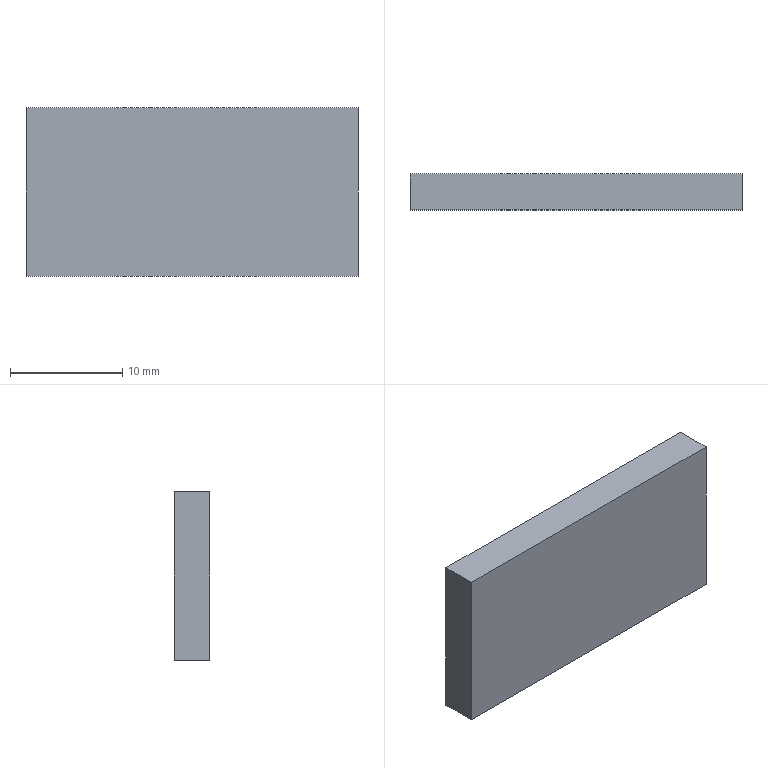Part | SolidWorks | features FlatPattern 1, SMBaseFlange 1, SheetMetal 1 | 1 solid | 6 faces | box 29.6 x 3.2 x 15 mm | volume 1421 mm3 | plane 6
STEP:
#1=CARTESIAN_POINT('',(0.,0.,-15.));
#2=VERTEX_POINT('',#1);
#3=CARTESIAN_POINT('',(0.,0.,0.));
#4=VERTEX_POINT('',#3);
#5=CARTESIAN_POINT('',(0.,0.,0.));
#6=DIRECTION('',(0.,0.,1.));
#7=VECTOR('',#6,1000.);
#8=LINE('',#5,#7);
#9=EDGE_CURVE('',#2,#4,#8,.T.);
#10=ORIENTED_EDGE('',*,*,#9,.F.);
#11=CARTESIAN_POINT('',(0.,-3.2,-15.));
#12=VERTEX_POINT('',#11);
#13=CARTESIAN_POINT('',(0.,-3.2,-15.));
#14=DIRECTION('',(0.,1.,0.));
#15=VECTOR('',#14,1000.);
#16=LINE('',#13,#15);
#17=EDGE_CURVE('',#12,#2,#16,.T.);
#18=ORIENTED_EDGE('',*,*,#17,.F.);
#19=CARTESIAN_POINT('',(0.,-3.2,0.));
#20=VERTEX_POINT('',#19);
#21=CARTESIAN_POINT('',(0.,-3.2,0.));
#22=DIRECTION('',(0.,0.,1.));
#23=VECTOR('',#22,1000.);
#24=LINE('',#21,#23);
#25=EDGE_CURVE('',#12,#20,#24,.T.);
#26=ORIENTED_EDGE('',*,*,#25,.T.);
#27=CARTESIAN_POINT('',(0.,-3.2,0.));
#28=DIRECTION('',(0.,1.,0.));
#29=VECTOR('',#28,1000.);
#30=LINE('',#27,#29);
#31=EDGE_CURVE('',#20,#4,#30,.T.);
#32=ORIENTED_EDGE('',*,*,#31,.T.);
#33=EDGE_LOOP('',(#10,#18,#26,#32));
#34=FACE_OUTER_BOUND('',#33,.T.);
#35=CARTESIAN_POINT('',(0.,-3.2,0.));
#36=DIRECTION('',(-1.,0.,0.));
#37=DIRECTION('',(0.,0.,1.));
#38=AXIS2_PLACEMENT_3D('',#35,#36,#37);
#39=PLANE('',#38);
#40=ADVANCED_FACE('',(#34),#39,.T.);
#41=CARTESIAN_POINT('',(29.6,0.,-15.));
#42=VERTEX_POINT('',#41);
#43=CARTESIAN_POINT('',(0.,0.,-15.));
#44=DIRECTION('',(-1.,0.,0.));
#45=VECTOR('',#44,1000.);
#46=LINE('',#43,#45);
#47=EDGE_CURVE('',#42,#2,#46,.T.);
#48=ORIENTED_EDGE('',*,*,#47,.F.);
#49=CARTESIAN_POINT('',(29.6,-3.2,-15.));
#50=VERTEX_POINT('',#49);
#51=CARTESIAN_POINT('',(29.6,-3.2,-15.));
#52=DIRECTION('',(0.,1.,0.));
#53=VECTOR('',#52,1000.);
#54=LINE('',#51,#53);
#55=EDGE_CURVE('',#50,#42,#54,.T.);
#56=ORIENTED_EDGE('',*,*,#55,.F.);
#57=CARTESIAN_POINT('',(0.,-3.2,-15.));
#58=DIRECTION('',(-1.,0.,0.));
#59=VECTOR('',#58,1000.);
#60=LINE('',#57,#59);
#61=EDGE_CURVE('',#50,#12,#60,.T.);
#62=ORIENTED_EDGE('',*,*,#61,.T.);
#63=ORIENTED_EDGE('',*,*,#17,.T.);
#64=EDGE_LOOP('',(#48,#56,#62,#63));
#65=FACE_OUTER_BOUND('',#64,.T.);
#66=CARTESIAN_POINT('',(0.,-3.2,-15.));
#67=DIRECTION('',(0.,0.,-1.));
#68=DIRECTION('',(-1.,0.,0.));
#69=AXIS2_PLACEMENT_3D('',#66,#67,#68);
#70=PLANE('',#69);
#71=ADVANCED_FACE('',(#65),#70,.T.);
#72=CARTESIAN_POINT('',(29.6,0.,0.));
#73=VERTEX_POINT('',#72);
#74=CARTESIAN_POINT('',(29.6,0.,0.));
#75=DIRECTION('',(0.,0.,-1.));
#76=VECTOR('',#75,1000.);
#77=LINE('',#74,#76);
#78=EDGE_CURVE('',#73,#42,#77,.T.);
#79=ORIENTED_EDGE('',*,*,#78,.F.);
#80=CARTESIAN_POINT('',(29.6,-3.2,0.));
#81=VERTEX_POINT('',#80);
#82=CARTESIAN_POINT('',(29.6,-3.2,0.));
#83=DIRECTION('',(0.,1.,0.));
#84=VECTOR('',#83,1000.);
#85=LINE('',#82,#84);
#86=EDGE_CURVE('',#81,#73,#85,.T.);
#87=ORIENTED_EDGE('',*,*,#86,.F.);
#88=CARTESIAN_POINT('',(29.6,-3.2,0.));
#89=DIRECTION('',(0.,0.,-1.));
#90=VECTOR('',#89,1000.);
#91=LINE('',#88,#90);
#92=EDGE_CURVE('',#81,#50,#91,.T.);
#93=ORIENTED_EDGE('',*,*,#92,.T.);
#94=ORIENTED_EDGE('',*,*,#55,.T.);
#95=EDGE_LOOP('',(#79,#87,#93,#94));
#96=FACE_OUTER_BOUND('',#95,.T.);
#97=CARTESIAN_POINT('',(29.6,-3.2,0.));
#98=DIRECTION('',(1.,0.,0.));
#99=DIRECTION('',(0.,0.,-1.));
#100=AXIS2_PLACEMENT_3D('',#97,#98,#99);
#101=PLANE('',#100);
#102=ADVANCED_FACE('',(#96),#101,.T.);
#103=CARTESIAN_POINT('',(0.,0.,0.));
#104=DIRECTION('',(1.,0.,0.));
#105=VECTOR('',#104,1000.);
#106=LINE('',#103,#105);
#107=EDGE_CURVE('',#4,#73,#106,.T.);
#108=ORIENTED_EDGE('',*,*,#107,.F.);
#109=ORIENTED_EDGE('',*,*,#31,.F.);
#110=CARTESIAN_POINT('',(0.,-3.2,0.));
#111=DIRECTION('',(1.,0.,0.));
#112=VECTOR('',#111,1000.);
#113=LINE('',#110,#112);
#114=EDGE_CURVE('',#20,#81,#113,.T.);
#115=ORIENTED_EDGE('',*,*,#114,.T.);
#116=ORIENTED_EDGE('',*,*,#86,.T.);
#117=EDGE_LOOP('',(#108,#109,#115,#116));
#118=FACE_OUTER_BOUND('',#117,.T.);
#119=CARTESIAN_POINT('',(0.,-3.2,0.));
#120=DIRECTION('',(0.,0.,1.));
#121=DIRECTION('',(1.,0.,0.));
#122=AXIS2_PLACEMENT_3D('',#119,#120,#121);
#123=PLANE('',#122);
#124=ADVANCED_FACE('',(#118),#123,.T.);
#125=ORIENTED_EDGE('',*,*,#25,.F.);
#126=ORIENTED_EDGE('',*,*,#61,.F.);
#127=ORIENTED_EDGE('',*,*,#92,.F.);
#128=ORIENTED_EDGE('',*,*,#114,.F.);
#129=EDGE_LOOP('',(#125,#126,#127,#128));
#130=FACE_OUTER_BOUND('',#129,.T.);
#131=CARTESIAN_POINT('',(0.,-3.2,0.));
#132=DIRECTION('',(0.,-1.,0.));
#133=DIRECTION('',(0.,0.,-1.));
#134=AXIS2_PLACEMENT_3D('',#131,#132,#133);
#135=PLANE('',#134);
#136=ADVANCED_FACE('',(#130),#135,.T.);
#137=ORIENTED_EDGE('',*,*,#9,.T.);
#138=ORIENTED_EDGE('',*,*,#107,.T.);
#139=ORIENTED_EDGE('',*,*,#78,.T.);
#140=ORIENTED_EDGE('',*,*,#47,.T.);
#141=EDGE_LOOP('',(#137,#138,#139,#140));
#142=FACE_OUTER_BOUND('',#141,.T.);
#143=CARTESIAN_POINT('',(0.,0.,0.));
#144=DIRECTION('',(0.,-1.,0.));
#145=DIRECTION('',(0.,0.,-1.));
#146=AXIS2_PLACEMENT_3D('',#143,#144,#145);
#147=PLANE('',#146);
#148=ADVANCED_FACE('',(#142),#147,.F.);
#149=CLOSED_SHELL('',(#40,#71,#102,#124,#136,#148));
#150=MANIFOLD_SOLID_BREP('',#149);
#151=CARTESIAN_POINT('',(0.,0.,0.));
#152=DIRECTION('',(0.,0.,1.));
#153=DIRECTION('',(1.,0.,0.));
#154=AXIS2_PLACEMENT_3D('',#151,#152,#153);
#155=(LENGTH_UNIT()NAMED_UNIT(*)SI_UNIT(.MILLI.,.METRE.));
#156=UNCERTAINTY_MEASURE_WITH_UNIT(LENGTH_MEASURE(0.00001),#155,'','');
#157=(NAMED_UNIT(*)PLANE_ANGLE_UNIT()SI_UNIT($,.RADIAN.));
#158=(NAMED_UNIT(*)SI_UNIT($,.STERADIAN.)SOLID_ANGLE_UNIT());
#159=(GEOMETRIC_REPRESENTATION_CONTEXT(3)GLOBAL_UNCERTAINTY_ASSIGNED_CONTEXT((#156))GLOBAL_UNIT_ASSIGNED_CONTEXT((#155,#157,#158))REPRESENTATION_CONTEXT('',''));
#160=ADVANCED_BREP_SHAPE_REPRESENTATION('',(#150,#154),#159);